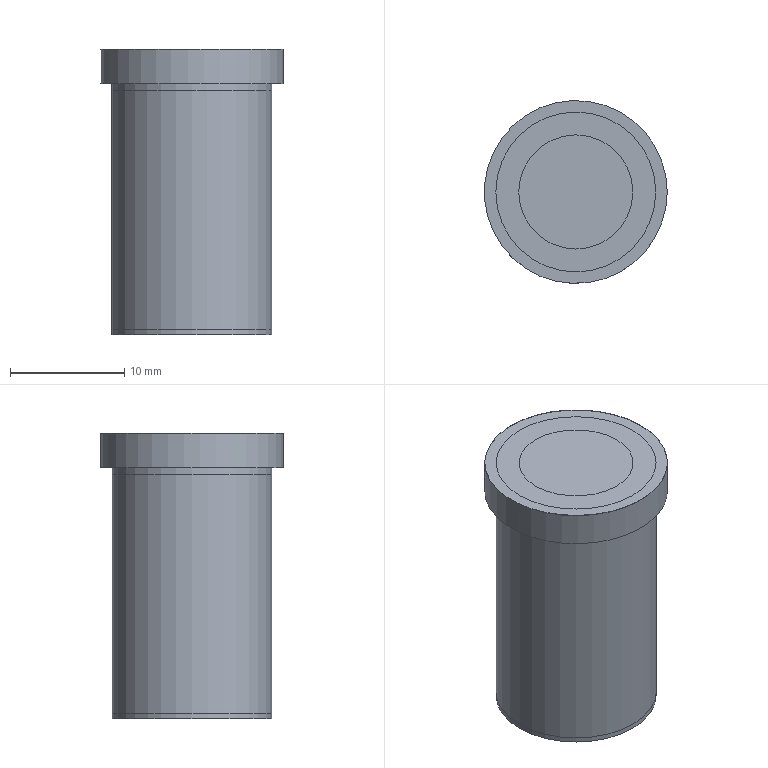Part | NX | features BREP 2 | 2 solids | 16 faces | box 16 x 16 x 25.03 mm | volume 6008 mm3 | plane 8 | cylinder 7 | cone 1 | commonest cylinder face diameters 14 x3 16 x2 10 x1 13.533 x1
STEP:
#1=CARTESIAN_POINT('',(8.,0.,-3.03));
#2=VERTEX_POINT('',#1);
#3=CARTESIAN_POINT('',(0.,0.,-3.03));
#4=DIRECTION('',(0.,0.,1.));
#5=DIRECTION('',(1.,0.,0.));
#6=AXIS2_PLACEMENT_3D('',#3,#4,#5);
#7=CIRCLE('',#6,8.);
#8=EDGE_CURVE('',#2,#2,#7,.T.);
#9=ORIENTED_EDGE('',*,*,#8,.T.);
#10=EDGE_LOOP('',(#9));
#11=FACE_BOUND('',#10,.T.);
#12=CARTESIAN_POINT('',(8.,0.,0.));
#13=VERTEX_POINT('',#12);
#14=CARTESIAN_POINT('',(0.,0.,0.));
#15=DIRECTION('',(0.,0.,1.));
#16=DIRECTION('',(1.,0.,0.));
#17=AXIS2_PLACEMENT_3D('',#14,#15,#16);
#18=CIRCLE('',#17,8.);
#19=EDGE_CURVE('',#13,#13,#18,.T.);
#20=ORIENTED_EDGE('',*,*,#19,.F.);
#21=EDGE_LOOP('',(#20));
#22=FACE_BOUND('',#21,.T.);
#23=CARTESIAN_POINT('',(0.,0.,-3.03));
#24=DIRECTION('',(0.,0.,1.));
#25=DIRECTION('',(-1.,0.,0.));
#26=AXIS2_PLACEMENT_3D('',#23,#24,#25);
#27=CYLINDRICAL_SURFACE('',#26,8.);
#28=ADVANCED_FACE('',(#11,#22),#27,.T.);
#29=CARTESIAN_POINT('',(-7.,0.,-3.03));
#30=VERTEX_POINT('',#29);
#31=CARTESIAN_POINT('',(0.,0.,-3.03));
#32=DIRECTION('',(0.,0.,-1.));
#33=DIRECTION('',(-1.,0.,0.));
#34=AXIS2_PLACEMENT_3D('',#31,#32,#33);
#35=CIRCLE('',#34,7.);
#36=EDGE_CURVE('',#30,#30,#35,.T.);
#37=ORIENTED_EDGE('',*,*,#36,.F.);
#38=EDGE_LOOP('',(#37));
#39=FACE_BOUND('',#38,.T.);
#40=ORIENTED_EDGE('',*,*,#8,.F.);
#41=EDGE_LOOP('',(#40));
#42=FACE_BOUND('',#41,.T.);
#43=CARTESIAN_POINT('',(0.,0.,-3.03));
#44=DIRECTION('',(0.,0.,1.));
#45=DIRECTION('',(-1.,0.,0.));
#46=AXIS2_PLACEMENT_3D('',#43,#44,#45);
#47=PLANE('',#46);
#48=ADVANCED_FACE('',(#39,#42),#47,.F.);
#49=ORIENTED_EDGE('',*,*,#19,.T.);
#50=EDGE_LOOP('',(#49));
#51=FACE_BOUND('',#50,.T.);
#52=CARTESIAN_POINT('',(0.,0.,0.));
#53=DIRECTION('',(0.,0.,1.));
#54=DIRECTION('',(-1.,0.,0.));
#55=AXIS2_PLACEMENT_3D('',#52,#53,#54);
#56=PLANE('',#55);
#57=ADVANCED_FACE('',(#51),#56,.T.);
#58=CARTESIAN_POINT('',(-7.,0.,-25.));
#59=VERTEX_POINT('',#58);
#60=CARTESIAN_POINT('',(0.,0.,-25.));
#61=DIRECTION('',(0.,0.,-1.));
#62=DIRECTION('',(-1.,0.,0.));
#63=AXIS2_PLACEMENT_3D('',#60,#61,#62);
#64=CIRCLE('',#63,7.);
#65=EDGE_CURVE('',#59,#59,#64,.T.);
#66=ORIENTED_EDGE('',*,*,#65,.T.);
#67=EDGE_LOOP('',(#66));
#68=FACE_BOUND('',#67,.T.);
#69=CARTESIAN_POINT('',(0.,0.,-25.));
#70=DIRECTION('',(0.,0.,-1.));
#71=DIRECTION('',(1.,0.,0.));
#72=AXIS2_PLACEMENT_3D('',#69,#70,#71);
#73=PLANE('',#72);
#74=ADVANCED_FACE('',(#68),#73,.T.);
#75=ORIENTED_EDGE('',*,*,#65,.F.);
#76=EDGE_LOOP('',(#75));
#77=FACE_BOUND('',#76,.T.);
#78=ORIENTED_EDGE('',*,*,#36,.T.);
#79=EDGE_LOOP('',(#78));
#80=FACE_BOUND('',#79,.T.);
#81=CARTESIAN_POINT('',(0.,0.,-3.03));
#82=DIRECTION('',(0.,0.,-1.));
#83=DIRECTION('',(1.,0.,0.));
#84=AXIS2_PLACEMENT_3D('',#81,#82,#83);
#85=CYLINDRICAL_SURFACE('',#84,7.);
#86=ADVANCED_FACE('',(#77,#80),#85,.T.);
#87=CLOSED_SHELL('',(#28,#48,#57,#74,#86));
#88=MANIFOLD_SOLID_BREP('',#87);
#89=CARTESIAN_POINT('',(-6.533,0.,-25.03));
#90=VERTEX_POINT('',#89);
#91=CARTESIAN_POINT('',(0.,0.,-25.03));
#92=DIRECTION('',(0.,0.,-1.));
#93=DIRECTION('',(-1.,0.,0.));
#94=AXIS2_PLACEMENT_3D('',#91,#92,#93);
#95=CIRCLE('',#94,6.533);
#96=EDGE_CURVE('',#90,#90,#95,.T.);
#97=ORIENTED_EDGE('',*,*,#96,.T.);
#98=EDGE_LOOP('',(#97));
#99=FACE_BOUND('',#98,.T.);
#100=CARTESIAN_POINT('',(5.,0.,-25.03));
#101=VERTEX_POINT('',#100);
#102=CARTESIAN_POINT('',(0.,0.,-25.03));
#103=DIRECTION('',(0.,0.,1.));
#104=DIRECTION('',(1.,0.,0.));
#105=AXIS2_PLACEMENT_3D('',#102,#103,#104);
#106=CIRCLE('',#105,5.);
#107=EDGE_CURVE('',#101,#101,#106,.T.);
#108=ORIENTED_EDGE('',*,*,#107,.T.);
#109=EDGE_LOOP('',(#108));
#110=FACE_BOUND('',#109,.T.);
#111=CARTESIAN_POINT('',(0.,0.,-25.03));
#112=DIRECTION('',(0.,0.,-1.));
#113=DIRECTION('',(1.,0.,0.));
#114=AXIS2_PLACEMENT_3D('',#111,#112,#113);
#115=PLANE('',#114);
#116=ADVANCED_FACE('',(#99,#110),#115,.T.);
#117=CARTESIAN_POINT('',(7.,0.,-0.026));
#118=VERTEX_POINT('',#117);
#119=CARTESIAN_POINT('',(0.,0.,-0.026));
#120=DIRECTION('',(0.,0.,1.));
#121=DIRECTION('',(1.,0.,0.));
#122=AXIS2_PLACEMENT_3D('',#119,#120,#121);
#123=CIRCLE('',#122,7.);
#124=EDGE_CURVE('',#118,#118,#123,.T.);
#125=ORIENTED_EDGE('',*,*,#124,.T.);
#126=EDGE_LOOP('',(#125));
#127=FACE_BOUND('',#126,.T.);
#128=CARTESIAN_POINT('',(5.,0.,-0.026));
#129=VERTEX_POINT('',#128);
#130=CARTESIAN_POINT('',(0.,0.,-0.026));
#131=DIRECTION('',(0.,0.,1.));
#132=DIRECTION('',(1.,0.,0.));
#133=AXIS2_PLACEMENT_3D('',#130,#131,#132);
#134=CIRCLE('',#133,5.);
#135=EDGE_CURVE('',#129,#129,#134,.T.);
#136=ORIENTED_EDGE('',*,*,#135,.F.);
#137=EDGE_LOOP('',(#136));
#138=FACE_BOUND('',#137,.T.);
#139=CARTESIAN_POINT('',(0.,0.,-0.026));
#140=DIRECTION('',(0.,0.,1.));
#141=DIRECTION('',(-1.,0.,0.));
#142=AXIS2_PLACEMENT_3D('',#139,#140,#141);
#143=PLANE('',#142);
#144=ADVANCED_FACE('',(#127,#138),#143,.T.);
#145=CARTESIAN_POINT('',(8.,0.,-3.03));
#146=VERTEX_POINT('',#145);
#147=CARTESIAN_POINT('',(0.,0.,-3.03));
#148=DIRECTION('',(0.,0.,1.));
#149=DIRECTION('',(1.,0.,0.));
#150=AXIS2_PLACEMENT_3D('',#147,#148,#149);
#151=CIRCLE('',#150,8.);
#152=EDGE_CURVE('',#146,#146,#151,.T.);
#153=ORIENTED_EDGE('',*,*,#152,.T.);
#154=EDGE_LOOP('',(#153));
#155=FACE_BOUND('',#154,.T.);
#156=CARTESIAN_POINT('',(8.,0.,-0.03));
#157=VERTEX_POINT('',#156);
#158=CARTESIAN_POINT('',(0.,0.,-0.03));
#159=DIRECTION('',(0.,0.,1.));
#160=DIRECTION('',(1.,0.,0.));
#161=AXIS2_PLACEMENT_3D('',#158,#159,#160);
#162=CIRCLE('',#161,8.);
#163=EDGE_CURVE('',#157,#157,#162,.T.);
#164=ORIENTED_EDGE('',*,*,#163,.F.);
#165=EDGE_LOOP('',(#164));
#166=FACE_BOUND('',#165,.T.);
#167=CARTESIAN_POINT('',(0.,0.,-3.03));
#168=DIRECTION('',(0.,0.,1.));
#169=DIRECTION('',(-1.,0.,0.));
#170=AXIS2_PLACEMENT_3D('',#167,#168,#169);
#171=CYLINDRICAL_SURFACE('',#170,8.);
#172=ADVANCED_FACE('',(#155,#166),#171,.T.);
#173=ORIENTED_EDGE('',*,*,#152,.F.);
#174=EDGE_LOOP('',(#173));
#175=FACE_BOUND('',#174,.T.);
#176=CARTESIAN_POINT('',(-6.767,0.,-3.03));
#177=VERTEX_POINT('',#176);
#178=CARTESIAN_POINT('',(0.,0.,-3.03));
#179=DIRECTION('',(0.,0.,-1.));
#180=DIRECTION('',(-1.,0.,0.));
#181=AXIS2_PLACEMENT_3D('',#178,#179,#180);
#182=CIRCLE('',#181,6.767);
#183=EDGE_CURVE('',#177,#177,#182,.T.);
#184=ORIENTED_EDGE('',*,*,#183,.F.);
#185=EDGE_LOOP('',(#184));
#186=FACE_BOUND('',#185,.T.);
#187=CARTESIAN_POINT('',(0.,0.,-3.03));
#188=DIRECTION('',(0.,0.,1.));
#189=DIRECTION('',(-1.,0.,0.));
#190=AXIS2_PLACEMENT_3D('',#187,#188,#189);
#191=PLANE('',#190);
#192=ADVANCED_FACE('',(#175,#186),#191,.F.);
#193=CARTESIAN_POINT('',(7.,0.,-0.03));
#194=VERTEX_POINT('',#193);
#195=CARTESIAN_POINT('',(0.,0.,-0.03));
#196=DIRECTION('',(0.,0.,1.));
#197=DIRECTION('',(1.,0.,0.));
#198=AXIS2_PLACEMENT_3D('',#195,#196,#197);
#199=CIRCLE('',#198,7.);
#200=EDGE_CURVE('',#194,#194,#199,.T.);
#201=ORIENTED_EDGE('',*,*,#200,.F.);
#202=EDGE_LOOP('',(#201));
#203=FACE_BOUND('',#202,.T.);
#204=ORIENTED_EDGE('',*,*,#163,.T.);
#205=EDGE_LOOP('',(#204));
#206=FACE_BOUND('',#205,.T.);
#207=CARTESIAN_POINT('',(0.,0.,-0.03));
#208=DIRECTION('',(0.,0.,1.));
#209=DIRECTION('',(-1.,0.,0.));
#210=AXIS2_PLACEMENT_3D('',#207,#208,#209);
#211=PLANE('',#210);
#212=ADVANCED_FACE('',(#203,#206),#211,.T.);
#213=CARTESIAN_POINT('',(-7.,0.,-24.563));
#214=VERTEX_POINT('',#213);
#215=CARTESIAN_POINT('',(0.,0.,-24.563));
#216=DIRECTION('',(0.,0.,1.));
#217=DIRECTION('',(-1.,0.,0.));
#218=AXIS2_PLACEMENT_3D('',#215,#216,#217);
#219=CIRCLE('',#218,7.);
#220=EDGE_CURVE('',#214,#214,#219,.T.);
#221=ORIENTED_EDGE('',*,*,#220,.T.);
#222=EDGE_LOOP('',(#221));
#223=FACE_BOUND('',#222,.T.);
#224=CARTESIAN_POINT('',(-7.,0.,-3.59));
#225=VERTEX_POINT('',#224);
#226=CARTESIAN_POINT('',(0.,0.,-3.59));
#227=DIRECTION('',(0.,0.,1.));
#228=DIRECTION('',(-1.,0.,0.));
#229=AXIS2_PLACEMENT_3D('',#226,#227,#228);
#230=CIRCLE('',#229,7.);
#231=EDGE_CURVE('',#225,#225,#230,.T.);
#232=ORIENTED_EDGE('',*,*,#231,.F.);
#233=EDGE_LOOP('',(#232));
#234=FACE_BOUND('',#233,.T.);
#235=CARTESIAN_POINT('',(0.,0.,-3.03));
#236=DIRECTION('',(0.,0.,-1.));
#237=DIRECTION('',(1.,0.,0.));
#238=AXIS2_PLACEMENT_3D('',#235,#236,#237);
#239=CYLINDRICAL_SURFACE('',#238,7.);
#240=ADVANCED_FACE('',(#223,#234),#239,.T.);
#241=ORIENTED_EDGE('',*,*,#124,.F.);
#242=EDGE_LOOP('',(#241));
#243=FACE_BOUND('',#242,.T.);
#244=ORIENTED_EDGE('',*,*,#200,.T.);
#245=EDGE_LOOP('',(#244));
#246=FACE_BOUND('',#245,.T.);
#247=CARTESIAN_POINT('',(0.,0.,-0.03));
#248=DIRECTION('',(0.,0.,1.));
#249=DIRECTION('',(-1.,0.,0.));
#250=AXIS2_PLACEMENT_3D('',#247,#248,#249);
#251=CYLINDRICAL_SURFACE('',#250,7.);
#252=ADVANCED_FACE('',(#243,#246),#251,.T.);
#253=ORIENTED_EDGE('',*,*,#135,.T.);
#254=EDGE_LOOP('',(#253));
#255=FACE_BOUND('',#254,.T.);
#256=ORIENTED_EDGE('',*,*,#107,.F.);
#257=EDGE_LOOP('',(#256));
#258=FACE_BOUND('',#257,.T.);
#259=CARTESIAN_POINT('',(0.,0.,-0.026));
#260=DIRECTION('',(0.,0.,-1.));
#261=DIRECTION('',(1.,0.,0.));
#262=AXIS2_PLACEMENT_3D('',#259,#260,#261);
#263=CYLINDRICAL_SURFACE('',#262,5.);
#264=ADVANCED_FACE('',(#255,#258),#263,.F.);
#265=CARTESIAN_POINT('',(-6.767,0.,-3.59));
#266=VERTEX_POINT('',#265);
#267=CARTESIAN_POINT('',(0.,0.,-3.59));
#268=DIRECTION('',(0.,0.,-1.));
#269=DIRECTION('',(-1.,0.,0.));
#270=AXIS2_PLACEMENT_3D('',#267,#268,#269);
#271=CIRCLE('',#270,6.767);
#272=EDGE_CURVE('',#266,#266,#271,.T.);
#273=ORIENTED_EDGE('',*,*,#272,.F.);
#274=EDGE_LOOP('',(#273));
#275=FACE_BOUND('',#274,.T.);
#276=ORIENTED_EDGE('',*,*,#183,.T.);
#277=EDGE_LOOP('',(#276));
#278=FACE_BOUND('',#277,.T.);
#279=CARTESIAN_POINT('',(0.,0.,-3.31));
#280=DIRECTION('',(0.,0.,-1.));
#281=DIRECTION('',(1.,0.,0.));
#282=AXIS2_PLACEMENT_3D('',#279,#280,#281);
#283=CYLINDRICAL_SURFACE('',#282,6.767);
#284=ADVANCED_FACE('',(#275,#278),#283,.T.);
#285=ORIENTED_EDGE('',*,*,#231,.T.);
#286=EDGE_LOOP('',(#285));
#287=FACE_BOUND('',#286,.T.);
#288=ORIENTED_EDGE('',*,*,#272,.T.);
#289=EDGE_LOOP('',(#288));
#290=FACE_BOUND('',#289,.T.);
#291=CARTESIAN_POINT('',(0.,0.,-3.59));
#292=DIRECTION('',(0.,0.,-1.));
#293=DIRECTION('',(1.,0.,0.));
#294=AXIS2_PLACEMENT_3D('',#291,#292,#293);
#295=PLANE('',#294);
#296=ADVANCED_FACE('',(#287,#290),#295,.F.);
#297=ORIENTED_EDGE('',*,*,#220,.F.);
#298=EDGE_LOOP('',(#297));
#299=FACE_BOUND('',#298,.T.);
#300=ORIENTED_EDGE('',*,*,#96,.F.);
#301=EDGE_LOOP('',(#300));
#302=FACE_BOUND('',#301,.T.);
#303=CARTESIAN_POINT('',(0.,0.,-25.03));
#304=DIRECTION('',(0.,0.,1.));
#305=DIRECTION('',(-1.,0.,0.));
#306=AXIS2_PLACEMENT_3D('',#303,#304,#305);
#307=CONICAL_SURFACE('',#306,6.533,0.7854);
#308=ADVANCED_FACE('',(#299,#302),#307,.T.);
#309=CLOSED_SHELL('',(#116,#144,#172,#192,#212,#240,#252,#264,#284,#296,#308));
#310=MANIFOLD_SOLID_BREP('',#309);
#311=(LENGTH_UNIT()NAMED_UNIT(*)SI_UNIT(.MILLI.,.METRE.));
#312=UNCERTAINTY_MEASURE_WITH_UNIT(LENGTH_MEASURE(0.00001),#311,'','');
#313=(NAMED_UNIT(*)PLANE_ANGLE_UNIT()SI_UNIT($,.RADIAN.));
#314=(NAMED_UNIT(*)SI_UNIT($,.STERADIAN.)SOLID_ANGLE_UNIT());
#315=(GEOMETRIC_REPRESENTATION_CONTEXT(3)GLOBAL_UNCERTAINTY_ASSIGNED_CONTEXT((#312))GLOBAL_UNIT_ASSIGNED_CONTEXT((#311,#313,#314))REPRESENTATION_CONTEXT('',''));
#316=ADVANCED_BREP_SHAPE_REPRESENTATION('',(#88,#310),#315);